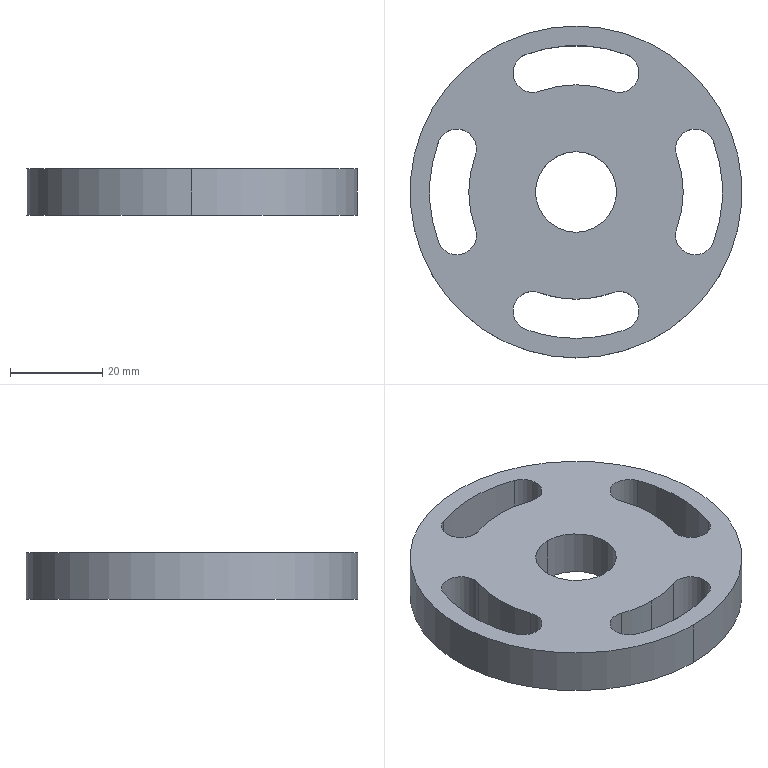CAM job | NX | 3-axis milling | part box 72 x 72 x 10 mm | stock box 72 x 72 x 10 mm
Tools:
number,name,description,diameter,corner_radius,flute_length,length,flutes
6,D6C,Milling Tool-5 Parameters,6.0,0.0,50.0,75.0,2
8,D6JING,Milling Tool-5 Parameters,6.0,0.0,50.0,75.0,2
7,D6A45,Milling Tool-5 Parameters,6.0,0.0,50.0,75.0,2
Operations:
program,operation,operation_type,tool,method,geometry_group,spindle_rpm,surface_speed,feed_per_tooth,feed_cut,feed_plunge,cut_length_mm,path_length_mm,cut_time_min,machine_time_min
1,ZLEVEL_PROFILE,ZLevelMilling,D6C,METHOD,A,4000.0,75.0,0.225,1800.0,100.0,40781.798,41187.784,22.657,22.697
1,ZLEVEL_PROFILE_COPY,ZLevelMilling,D6JING,METHOD,A,7500.0,141.0,0.0667,1000.0,100.0,210.53,677.07,0.2105,0.2572
1,PLANAR_MILL,PlanarMilling,D6A45,METHOD,A,7500.0,141.0,0.0833,1250.0,100.0,321.239,748.396,0.257,0.2997